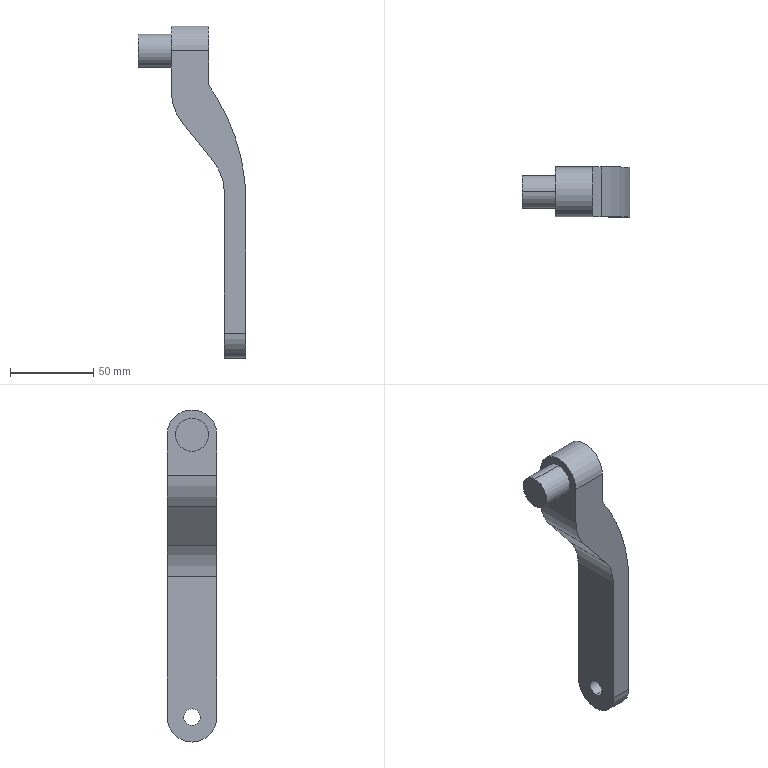Part | STEP file | Pedal LHS | 1 solid | 19 faces | box 65 x 30 x 200 mm | volume 107612 mm3 | cylinder 10 | plane 9 | commonest cylinder face diameters 30 x3 10 x2 20 x2 60 x2 240 x1
STEP:
#1=CARTESIAN_POINT('',(0.,0.,0.));
#2=DIRECTION('',(0.,0.,1.));
#3=DIRECTION('',(1.,0.,0.));
#4=AXIS2_PLACEMENT_3D('',#1,#2,#3);
#5=CARTESIAN_POINT('',(-65.,0.,10.));
#6=VERTEX_POINT('',#5);
#7=CARTESIAN_POINT('',(-65.,0.,-10.));
#8=VERTEX_POINT('',#7);
#9=CARTESIAN_POINT('',(-65.,0.,0.));
#10=DIRECTION('',(-1.,0.,0.));
#11=DIRECTION('',(0.,0.,1.));
#12=AXIS2_PLACEMENT_3D('',#9,#10,#11);
#13=CIRCLE('',#12,10.);
#14=CARTESIAN_POINT('',(-65.,0.,0.));
#15=DIRECTION('',(1.,0.,0.));
#16=DIRECTION('',(0.,0.,-1.));
#17=AXIS2_PLACEMENT_3D('',#14,#15,#16);
#18=CYLINDRICAL_SURFACE('',#17,10.);
#19=CARTESIAN_POINT('',(3.142,0.));
#20=DIRECTION('',(-1.,0.));
#21=VECTOR('',#20,1.);
#22=LINE('',#19,#21);
#23=(GEOMETRIC_REPRESENTATION_CONTEXT(2)PARAMETRIC_REPRESENTATION_CONTEXT()REPRESENTATION_CONTEXT('',''));
#24=DEFINITIONAL_REPRESENTATION('',(#22),#23);
#25=PCURVE('',#18,#24);
#26=CARTESIAN_POINT('',(-65.,0.,0.));
#27=DIRECTION('',(-1.,0.,0.));
#28=DIRECTION('',(0.,0.,1.));
#29=AXIS2_PLACEMENT_3D('',#26,#27,#28);
#30=PLANE('',#29);
#31=CARTESIAN_POINT('',(0.,0.));
#32=DIRECTION('',(1.,0.));
#33=AXIS2_PLACEMENT_2D('',#31,#32);
#34=CIRCLE('',#33,10.);
#35=(GEOMETRIC_REPRESENTATION_CONTEXT(2)PARAMETRIC_REPRESENTATION_CONTEXT()REPRESENTATION_CONTEXT('',''));
#36=DEFINITIONAL_REPRESENTATION('',(#34),#35);
#37=PCURVE('',#30,#36);
#38=SURFACE_CURVE('',#13,(#25,#37),.PCURVE_S1.);
#39=EDGE_CURVE('',#6,#8,#38,.T.);
#40=ORIENTED_EDGE('',*,*,#39,.F.);
#41=CARTESIAN_POINT('',(-45.,0.,10.));
#42=VERTEX_POINT('',#41);
#43=CARTESIAN_POINT('',(-65.,0.,10.));
#44=DIRECTION('',(1.,0.,0.));
#45=VECTOR('',#44,1.);
#46=LINE('',#43,#45);
#47=CARTESIAN_POINT('',(3.142,0.));
#48=DIRECTION('',(0.,1.));
#49=VECTOR('',#48,1.);
#50=LINE('',#47,#49);
#51=(GEOMETRIC_REPRESENTATION_CONTEXT(2)PARAMETRIC_REPRESENTATION_CONTEXT()REPRESENTATION_CONTEXT('',''));
#52=DEFINITIONAL_REPRESENTATION('',(#50),#51);
#53=PCURVE('',#18,#52);
#54=CARTESIAN_POINT('',(-65.,0.,0.));
#55=DIRECTION('',(1.,0.,0.));
#56=DIRECTION('',(0.,0.,-1.));
#57=AXIS2_PLACEMENT_3D('',#54,#55,#56);
#58=CYLINDRICAL_SURFACE('',#57,10.);
#59=CARTESIAN_POINT('',(3.142,0.));
#60=DIRECTION('',(0.,1.));
#61=VECTOR('',#60,1.);
#62=LINE('',#59,#61);
#63=(GEOMETRIC_REPRESENTATION_CONTEXT(2)PARAMETRIC_REPRESENTATION_CONTEXT()REPRESENTATION_CONTEXT('',''));
#64=DEFINITIONAL_REPRESENTATION('',(#62),#63);
#65=PCURVE('',#58,#64);
#66=SURFACE_CURVE('',#46,(#53,#65),.PCURVE_S1.);
#67=EDGE_CURVE('',#6,#42,#66,.T.);
#68=ORIENTED_EDGE('',*,*,#67,.T.);
#69=CARTESIAN_POINT('',(-45.,0.,-10.));
#70=VERTEX_POINT('',#69);
#71=CARTESIAN_POINT('',(-45.,0.,0.));
#72=DIRECTION('',(-1.,0.,0.));
#73=DIRECTION('',(0.,0.,-1.));
#74=AXIS2_PLACEMENT_3D('',#71,#72,#73);
#75=CIRCLE('',#74,10.);
#76=CARTESIAN_POINT('',(6.283,20.));
#77=DIRECTION('',(-1.,0.));
#78=VECTOR('',#77,1.);
#79=LINE('',#76,#78);
#80=(GEOMETRIC_REPRESENTATION_CONTEXT(2)PARAMETRIC_REPRESENTATION_CONTEXT()REPRESENTATION_CONTEXT('',''));
#81=DEFINITIONAL_REPRESENTATION('',(#79),#80);
#82=PCURVE('',#18,#81);
#83=CARTESIAN_POINT('',(-45.,0.,0.));
#84=DIRECTION('',(1.,0.,0.));
#85=DIRECTION('',(0.,0.,-1.));
#86=AXIS2_PLACEMENT_3D('',#83,#84,#85);
#87=PLANE('',#86);
#88=CARTESIAN_POINT('',(10.,0.));
#89=CARTESIAN_POINT('',(10.,-17.321));
#90=CARTESIAN_POINT('',(-5.,-8.66));
#91=CARTESIAN_POINT('',(-20.,0.));
#92=CARTESIAN_POINT('',(-5.,8.66));
#93=CARTESIAN_POINT('',(10.,17.321));
#94=CARTESIAN_POINT('',(10.,0.));
#95=(BOUNDED_CURVE()B_SPLINE_CURVE(2,(#88,#89,#90,#91,#92,#93,#94),.UNSPECIFIED.,.T.,.F.)B_SPLINE_CURVE_WITH_KNOTS((1,2,2,2,2,1),(-2.094,0.,2.094,4.189,6.283,8.378),.UNSPECIFIED.)CURVE()GEOMETRIC_REPRESENTATION_ITEM()RATIONAL_B_SPLINE_CURVE((1.,0.5,1.,0.5,1.,0.5,1.))REPRESENTATION_ITEM(''));
#96=(GEOMETRIC_REPRESENTATION_CONTEXT(2)PARAMETRIC_REPRESENTATION_CONTEXT()REPRESENTATION_CONTEXT('',''));
#97=DEFINITIONAL_REPRESENTATION('',(#95),#96);
#98=PCURVE('',#87,#97);
#99=SURFACE_CURVE('',#75,(#82,#98),.PCURVE_S1.);
#100=EDGE_CURVE('',#42,#70,#99,.T.);
#101=ORIENTED_EDGE('',*,*,#100,.T.);
#102=CARTESIAN_POINT('',(-65.,0.,-10.));
#103=DIRECTION('',(1.,0.,0.));
#104=VECTOR('',#103,1.);
#105=LINE('',#102,#104);
#106=CARTESIAN_POINT('',(0.,0.));
#107=DIRECTION('',(0.,1.));
#108=VECTOR('',#107,1.);
#109=LINE('',#106,#108);
#110=(GEOMETRIC_REPRESENTATION_CONTEXT(2)PARAMETRIC_REPRESENTATION_CONTEXT()REPRESENTATION_CONTEXT('',''));
#111=DEFINITIONAL_REPRESENTATION('',(#109),#110);
#112=PCURVE('',#18,#111);
#113=CARTESIAN_POINT('',(6.283,0.));
#114=DIRECTION('',(0.,1.));
#115=VECTOR('',#114,1.);
#116=LINE('',#113,#115);
#117=(GEOMETRIC_REPRESENTATION_CONTEXT(2)PARAMETRIC_REPRESENTATION_CONTEXT()REPRESENTATION_CONTEXT('',''));
#118=DEFINITIONAL_REPRESENTATION('',(#116),#117);
#119=PCURVE('',#58,#118);
#120=SURFACE_CURVE('',#105,(#112,#119),.PCURVE_S1.);
#121=EDGE_CURVE('',#8,#70,#120,.T.);
#122=ORIENTED_EDGE('',*,*,#121,.F.);
#123=EDGE_LOOP('',(#40,#68,#101,#122));
#124=FACE_BOUND('',#123,.T.);
#125=ADVANCED_FACE('',(#124),#18,.T.);
#126=CARTESIAN_POINT('',(-13.,0.,-175.));
#127=VERTEX_POINT('',#126);
#128=CARTESIAN_POINT('',(0.,0.,-175.));
#129=VERTEX_POINT('',#128);
#130=CARTESIAN_POINT('',(-45.,0.,-175.));
#131=DIRECTION('',(1.,0.,0.));
#132=VECTOR('',#131,1.);
#133=LINE('',#130,#132);
#134=CARTESIAN_POINT('',(-45.,0.,-170.));
#135=DIRECTION('',(1.,0.,0.));
#136=DIRECTION('',(0.,0.,-1.));
#137=AXIS2_PLACEMENT_3D('',#134,#135,#136);
#138=CYLINDRICAL_SURFACE('',#137,5.);
#139=CARTESIAN_POINT('',(6.283,0.));
#140=DIRECTION('',(0.,1.));
#141=VECTOR('',#140,1.);
#142=LINE('',#139,#141);
#143=(GEOMETRIC_REPRESENTATION_CONTEXT(2)PARAMETRIC_REPRESENTATION_CONTEXT()REPRESENTATION_CONTEXT('',''));
#144=DEFINITIONAL_REPRESENTATION('',(#142),#143);
#145=PCURVE('',#138,#144);
#146=CARTESIAN_POINT('',(-45.,0.,-170.));
#147=DIRECTION('',(1.,0.,0.));
#148=DIRECTION('',(0.,0.,-1.));
#149=AXIS2_PLACEMENT_3D('',#146,#147,#148);
#150=CYLINDRICAL_SURFACE('',#149,5.);
#151=CARTESIAN_POINT('',(0.,0.));
#152=DIRECTION('',(0.,1.));
#153=VECTOR('',#152,1.);
#154=LINE('',#151,#153);
#155=(GEOMETRIC_REPRESENTATION_CONTEXT(2)PARAMETRIC_REPRESENTATION_CONTEXT()REPRESENTATION_CONTEXT('',''));
#156=DEFINITIONAL_REPRESENTATION('',(#154),#155);
#157=PCURVE('',#150,#156);
#158=SURFACE_CURVE('',#133,(#145,#157),.PCURVE_S1.);
#159=EDGE_CURVE('',#127,#129,#158,.T.);
#160=ORIENTED_EDGE('',*,*,#159,.T.);
#161=CARTESIAN_POINT('',(0.,0.,-165.));
#162=VERTEX_POINT('',#161);
#163=CARTESIAN_POINT('',(0.,0.,-170.));
#164=DIRECTION('',(1.,0.,0.));
#165=DIRECTION('',(0.,0.,-1.));
#166=AXIS2_PLACEMENT_3D('',#163,#164,#165);
#167=CIRCLE('',#166,5.);
#168=CARTESIAN_POINT('',(0.,45.));
#169=DIRECTION('',(1.,0.));
#170=VECTOR('',#169,1.);
#171=LINE('',#168,#170);
#172=(GEOMETRIC_REPRESENTATION_CONTEXT(2)PARAMETRIC_REPRESENTATION_CONTEXT()REPRESENTATION_CONTEXT('',''));
#173=DEFINITIONAL_REPRESENTATION('',(#171),#172);
#174=PCURVE('',#138,#173);
#175=CARTESIAN_POINT('',(0.,0.,0.));
#176=DIRECTION('',(1.,0.,0.));
#177=DIRECTION('',(0.,0.,-1.));
#178=AXIS2_PLACEMENT_3D('',#175,#176,#177);
#179=PLANE('',#178);
#180=CARTESIAN_POINT('',(170.,0.));
#181=DIRECTION('',(1.,0.));
#182=AXIS2_PLACEMENT_2D('',#180,#181);
#183=CIRCLE('',#182,5.);
#184=(GEOMETRIC_REPRESENTATION_CONTEXT(2)PARAMETRIC_REPRESENTATION_CONTEXT()REPRESENTATION_CONTEXT('',''));
#185=DEFINITIONAL_REPRESENTATION('',(#183),#184);
#186=PCURVE('',#179,#185);
#187=SURFACE_CURVE('',#167,(#174,#186),.PCURVE_S1.);
#188=EDGE_CURVE('',#162,#129,#187,.T.);
#189=ORIENTED_EDGE('',*,*,#188,.F.);
#190=CARTESIAN_POINT('',(-13.,0.,-165.));
#191=VERTEX_POINT('',#190);
#192=CARTESIAN_POINT('',(-45.,0.,-165.));
#193=DIRECTION('',(1.,0.,0.));
#194=VECTOR('',#193,1.);
#195=LINE('',#192,#194);
#196=CARTESIAN_POINT('',(3.142,0.));
#197=DIRECTION('',(0.,1.));
#198=VECTOR('',#197,1.);
#199=LINE('',#196,#198);
#200=(GEOMETRIC_REPRESENTATION_CONTEXT(2)PARAMETRIC_REPRESENTATION_CONTEXT()REPRESENTATION_CONTEXT('',''));
#201=DEFINITIONAL_REPRESENTATION('',(#199),#200);
#202=PCURVE('',#138,#201);
#203=CARTESIAN_POINT('',(3.142,0.));
#204=DIRECTION('',(0.,1.));
#205=VECTOR('',#204,1.);
#206=LINE('',#203,#205);
#207=(GEOMETRIC_REPRESENTATION_CONTEXT(2)PARAMETRIC_REPRESENTATION_CONTEXT()REPRESENTATION_CONTEXT('',''));
#208=DEFINITIONAL_REPRESENTATION('',(#206),#207);
#209=PCURVE('',#150,#208);
#210=SURFACE_CURVE('',#195,(#202,#209),.PCURVE_S1.);
#211=EDGE_CURVE('',#191,#162,#210,.T.);
#212=ORIENTED_EDGE('',*,*,#211,.F.);
#213=CARTESIAN_POINT('',(-13.,0.,-170.));
#214=DIRECTION('',(1.,0.,0.));
#215=DIRECTION('',(0.,0.,1.));
#216=AXIS2_PLACEMENT_3D('',#213,#214,#215);
#217=CIRCLE('',#216,5.);
#218=CARTESIAN_POINT('',(3.142,32.));
#219=DIRECTION('',(1.,0.));
#220=VECTOR('',#219,1.);
#221=LINE('',#218,#220);
#222=(GEOMETRIC_REPRESENTATION_CONTEXT(2)PARAMETRIC_REPRESENTATION_CONTEXT()REPRESENTATION_CONTEXT('',''));
#223=DEFINITIONAL_REPRESENTATION('',(#221),#222);
#224=PCURVE('',#138,#223);
#225=CARTESIAN_POINT('',(-13.,-22.5,-185.));
#226=DIRECTION('',(-1.,0.,0.));
#227=DIRECTION('',(0.,0.,1.));
#228=AXIS2_PLACEMENT_3D('',#225,#226,#227);
#229=PLANE('',#228);
#230=CARTESIAN_POINT('',(20.,22.5));
#231=CARTESIAN_POINT('',(20.,13.84));
#232=CARTESIAN_POINT('',(12.5,18.17));
#233=CARTESIAN_POINT('',(5.,22.5));
#234=CARTESIAN_POINT('',(12.5,26.83));
#235=CARTESIAN_POINT('',(20.,31.16));
#236=CARTESIAN_POINT('',(20.,22.5));
#237=(BOUNDED_CURVE()B_SPLINE_CURVE(2,(#230,#231,#232,#233,#234,#235,#236),.UNSPECIFIED.,.T.,.F.)B_SPLINE_CURVE_WITH_KNOTS((1,2,2,2,2,1),(-2.094,0.,2.094,4.189,6.283,8.378),.UNSPECIFIED.)CURVE()GEOMETRIC_REPRESENTATION_ITEM()RATIONAL_B_SPLINE_CURVE((1.,0.5,1.,0.5,1.,0.5,1.))REPRESENTATION_ITEM(''));
#238=(GEOMETRIC_REPRESENTATION_CONTEXT(2)PARAMETRIC_REPRESENTATION_CONTEXT()REPRESENTATION_CONTEXT('',''));
#239=DEFINITIONAL_REPRESENTATION('',(#237),#238);
#240=PCURVE('',#229,#239);
#241=SURFACE_CURVE('',#217,(#224,#240),.PCURVE_S1.);
#242=EDGE_CURVE('',#191,#127,#241,.T.);
#243=ORIENTED_EDGE('',*,*,#242,.T.);
#244=EDGE_LOOP('',(#160,#189,#212,#243));
#245=FACE_BOUND('',#244,.F.);
#246=ADVANCED_FACE('',(#245),#138,.F.);
#247=CARTESIAN_POINT('',(-13.,-15.,-170.));
#248=VERTEX_POINT('',#247);
#249=CARTESIAN_POINT('',(-13.,0.,-185.));
#250=VERTEX_POINT('',#249);
#251=CARTESIAN_POINT('',(-13.,0.,-170.));
#252=DIRECTION('',(1.,0.,0.));
#253=DIRECTION('',(0.,0.,1.));
#254=AXIS2_PLACEMENT_3D('',#251,#252,#253);
#255=CIRCLE('',#254,15.);
#256=CARTESIAN_POINT('',(-45.,0.,-170.));
#257=DIRECTION('',(1.,0.,0.));
#258=DIRECTION('',(0.,0.,-1.));
#259=AXIS2_PLACEMENT_3D('',#256,#257,#258);
#260=CYLINDRICAL_SURFACE('',#259,15.);
#261=CARTESIAN_POINT('',(3.142,32.));
#262=DIRECTION('',(1.,0.));
#263=VECTOR('',#262,1.);
#264=LINE('',#261,#263);
#265=(GEOMETRIC_REPRESENTATION_CONTEXT(2)PARAMETRIC_REPRESENTATION_CONTEXT()REPRESENTATION_CONTEXT('',''));
#266=DEFINITIONAL_REPRESENTATION('',(#264),#265);
#267=PCURVE('',#260,#266);
#268=CARTESIAN_POINT('',(30.,22.5));
#269=CARTESIAN_POINT('',(30.,-3.481));
#270=CARTESIAN_POINT('',(7.5,9.51));
#271=CARTESIAN_POINT('',(-15.,22.5));
#272=CARTESIAN_POINT('',(7.5,35.49));
#273=CARTESIAN_POINT('',(30.,48.481));
#274=CARTESIAN_POINT('',(30.,22.5));
#275=(BOUNDED_CURVE()B_SPLINE_CURVE(2,(#268,#269,#270,#271,#272,#273,#274),.UNSPECIFIED.,.T.,.F.)B_SPLINE_CURVE_WITH_KNOTS((1,2,2,2,2,1),(-2.094,0.,2.094,4.189,6.283,8.378),.UNSPECIFIED.)CURVE()GEOMETRIC_REPRESENTATION_ITEM()RATIONAL_B_SPLINE_CURVE((1.,0.5,1.,0.5,1.,0.5,1.))REPRESENTATION_ITEM(''));
#276=(GEOMETRIC_REPRESENTATION_CONTEXT(2)PARAMETRIC_REPRESENTATION_CONTEXT()REPRESENTATION_CONTEXT('',''));
#277=DEFINITIONAL_REPRESENTATION('',(#275),#276);
#278=PCURVE('',#229,#277);
#279=SURFACE_CURVE('',#255,(#267,#278),.PCURVE_S1.);
#280=EDGE_CURVE('',#248,#250,#279,.T.);
#281=ORIENTED_EDGE('',*,*,#280,.T.);
#282=CARTESIAN_POINT('',(0.,0.,-185.));
#283=VERTEX_POINT('',#282);
#284=CARTESIAN_POINT('',(-45.,0.,-185.));
#285=DIRECTION('',(1.,0.,0.));
#286=VECTOR('',#285,1.);
#287=LINE('',#284,#286);
#288=CARTESIAN_POINT('',(6.283,0.));
#289=DIRECTION('',(0.,1.));
#290=VECTOR('',#289,1.);
#291=LINE('',#288,#290);
#292=(GEOMETRIC_REPRESENTATION_CONTEXT(2)PARAMETRIC_REPRESENTATION_CONTEXT()REPRESENTATION_CONTEXT('',''));
#293=DEFINITIONAL_REPRESENTATION('',(#291),#292);
#294=PCURVE('',#260,#293);
#295=CARTESIAN_POINT('',(-45.,0.,-170.));
#296=DIRECTION('',(1.,0.,0.));
#297=DIRECTION('',(0.,0.,-1.));
#298=AXIS2_PLACEMENT_3D('',#295,#296,#297);
#299=CYLINDRICAL_SURFACE('',#298,15.);
#300=CARTESIAN_POINT('',(0.,0.));
#301=DIRECTION('',(0.,1.));
#302=VECTOR('',#301,1.);
#303=LINE('',#300,#302);
#304=(GEOMETRIC_REPRESENTATION_CONTEXT(2)PARAMETRIC_REPRESENTATION_CONTEXT()REPRESENTATION_CONTEXT('',''));
#305=DEFINITIONAL_REPRESENTATION('',(#303),#304);
#306=PCURVE('',#299,#305);
#307=SURFACE_CURVE('',#287,(#294,#306),.PCURVE_S1.);
#308=EDGE_CURVE('',#250,#283,#307,.T.);
#309=ORIENTED_EDGE('',*,*,#308,.T.);
#310=CARTESIAN_POINT('',(0.,-15.,-170.));
#311=VERTEX_POINT('',#310);
#312=CARTESIAN_POINT('',(0.,0.,-170.));
#313=DIRECTION('',(1.,0.,0.));
#314=DIRECTION('',(0.,0.,-1.));
#315=AXIS2_PLACEMENT_3D('',#312,#313,#314);
#316=CIRCLE('',#315,15.);
#317=CARTESIAN_POINT('',(0.,45.));
#318=DIRECTION('',(1.,0.));
#319=VECTOR('',#318,1.);
#320=LINE('',#317,#319);
#321=(GEOMETRIC_REPRESENTATION_CONTEXT(2)PARAMETRIC_REPRESENTATION_CONTEXT()REPRESENTATION_CONTEXT('',''));
#322=DEFINITIONAL_REPRESENTATION('',(#320),#321);
#323=PCURVE('',#260,#322);
#324=CARTESIAN_POINT('',(170.,0.));
#325=DIRECTION('',(1.,0.));
#326=AXIS2_PLACEMENT_2D('',#324,#325);
#327=CIRCLE('',#326,15.);
#328=(GEOMETRIC_REPRESENTATION_CONTEXT(2)PARAMETRIC_REPRESENTATION_CONTEXT()REPRESENTATION_CONTEXT('',''));
#329=DEFINITIONAL_REPRESENTATION('',(#327),#328);
#330=PCURVE('',#179,#329);
#331=SURFACE_CURVE('',#316,(#323,#330),.PCURVE_S1.);
#332=EDGE_CURVE('',#311,#283,#331,.T.);
#333=ORIENTED_EDGE('',*,*,#332,.F.);
#334=CARTESIAN_POINT('',(-45.,-15.,-170.));
#335=DIRECTION('',(1.,0.,0.));
#336=VECTOR('',#335,1.);
#337=LINE('',#334,#336);
#338=CARTESIAN_POINT('',(4.712,0.));
#339=DIRECTION('',(0.,1.));
#340=VECTOR('',#339,1.);
#341=LINE('',#338,#340);
#342=(GEOMETRIC_REPRESENTATION_CONTEXT(2)PARAMETRIC_REPRESENTATION_CONTEXT()REPRESENTATION_CONTEXT('',''));
#343=DEFINITIONAL_REPRESENTATION('',(#341),#342);
#344=PCURVE('',#260,#343);
#345=CARTESIAN_POINT('',(-45.,-15.,0.));
#346=DIRECTION('',(0.,-1.,0.));
#347=DIRECTION('',(0.,0.,-1.));
#348=AXIS2_PLACEMENT_3D('',#345,#346,#347);
#349=PLANE('',#348);
#350=CARTESIAN_POINT('',(170.,0.));
#351=DIRECTION('',(0.,1.));
#352=VECTOR('',#351,1.);
#353=LINE('',#350,#352);
#354=(GEOMETRIC_REPRESENTATION_CONTEXT(2)PARAMETRIC_REPRESENTATION_CONTEXT()REPRESENTATION_CONTEXT('',''));
#355=DEFINITIONAL_REPRESENTATION('',(#353),#354);
#356=PCURVE('',#349,#355);
#357=SURFACE_CURVE('',#337,(#344,#356),.PCURVE_S1.);
#358=EDGE_CURVE('',#248,#311,#357,.T.);
#359=ORIENTED_EDGE('',*,*,#358,.F.);
#360=EDGE_LOOP('',(#281,#309,#333,#359));
#361=FACE_BOUND('',#360,.T.);
#362=ADVANCED_FACE('',(#361),#260,.T.);
#363=CARTESIAN_POINT('',(-45.,15.,-24.477));
#364=VERTEX_POINT('',#363);
#365=CARTESIAN_POINT('',(-45.,15.,0.));
#366=VERTEX_POINT('',#365);
#367=CARTESIAN_POINT('',(-45.,15.,0.));
#368=DIRECTION('',(0.,0.,1.));
#369=VECTOR('',#368,1.);
#370=LINE('',#367,#369);
#371=CARTESIAN_POINT('',(0.,15.));
#372=DIRECTION('',(-1.,0.));
#373=VECTOR('',#372,1.);
#374=LINE('',#371,#373);
#375=(GEOMETRIC_REPRESENTATION_CONTEXT(2)PARAMETRIC_REPRESENTATION_CONTEXT()REPRESENTATION_CONTEXT('',''));
#376=DEFINITIONAL_REPRESENTATION('',(#374),#375);
#377=PCURVE('',#87,#376);
#378=CARTESIAN_POINT('',(-45.,15.,0.));
#379=DIRECTION('',(0.,1.,0.));
#380=DIRECTION('',(0.,0.,1.));
#381=AXIS2_PLACEMENT_3D('',#378,#379,#380);
#382=PLANE('',#381);
#383=CARTESIAN_POINT('',(0.,0.));
#384=DIRECTION('',(1.,0.));
#385=VECTOR('',#384,1.);
#386=LINE('',#383,#385);
#387=(GEOMETRIC_REPRESENTATION_CONTEXT(2)PARAMETRIC_REPRESENTATION_CONTEXT()REPRESENTATION_CONTEXT('',''));
#388=DEFINITIONAL_REPRESENTATION('',(#386),#387);
#389=PCURVE('',#382,#388);
#390=SURFACE_CURVE('',#370,(#377,#389),.PCURVE_S1.);
#391=EDGE_CURVE('',#364,#366,#390,.T.);
#392=ORIENTED_EDGE('',*,*,#391,.F.);
#393=CARTESIAN_POINT('',(-45.,-15.,-24.477));
#394=VERTEX_POINT('',#393);
#395=CARTESIAN_POINT('',(-45.,-15.,-24.477));
#396=DIRECTION('',(0.,-1.,0.));
#397=VECTOR('',#396,1.);
#398=LINE('',#395,#397);
#399=CARTESIAN_POINT('',(24.477,-15.));
#400=DIRECTION('',(0.,-1.));
#401=VECTOR('',#400,1.);
#402=LINE('',#399,#401);
#403=(GEOMETRIC_REPRESENTATION_CONTEXT(2)PARAMETRIC_REPRESENTATION_CONTEXT()REPRESENTATION_CONTEXT('',''));
#404=DEFINITIONAL_REPRESENTATION('',(#402),#403);
#405=PCURVE('',#87,#404);
#406=CARTESIAN_POINT('',(-15.,-22.5,-24.477));
#407=DIRECTION('',(0.,-1.,0.));
#408=DIRECTION('',(0.,0.,-1.));
#409=AXIS2_PLACEMENT_3D('',#406,#407,#408);
#410=CYLINDRICAL_SURFACE('',#409,30.);
#411=CARTESIAN_POINT('',(4.712,-7.5));
#412=DIRECTION('',(0.,1.));
#413=VECTOR('',#412,1.);
#414=LINE('',#411,#413);
#415=(GEOMETRIC_REPRESENTATION_CONTEXT(2)PARAMETRIC_REPRESENTATION_CONTEXT()REPRESENTATION_CONTEXT('',''));
#416=DEFINITIONAL_REPRESENTATION('',(#414),#415);
#417=PCURVE('',#410,#416);
#418=SURFACE_CURVE('',#398,(#405,#417),.PCURVE_S1.);
#419=EDGE_CURVE('',#364,#394,#418,.T.);
#420=ORIENTED_EDGE('',*,*,#419,.T.);
#421=CARTESIAN_POINT('',(-45.,-15.,0.));
#422=VERTEX_POINT('',#421);
#423=CARTESIAN_POINT('',(-45.,-15.,0.));
#424=DIRECTION('',(0.,0.,-1.));
#425=VECTOR('',#424,1.);
#426=LINE('',#423,#425);
#427=CARTESIAN_POINT('',(0.,-15.));
#428=DIRECTION('',(1.,0.));
#429=VECTOR('',#428,1.);
#430=LINE('',#427,#429);
#431=(GEOMETRIC_REPRESENTATION_CONTEXT(2)PARAMETRIC_REPRESENTATION_CONTEXT()REPRESENTATION_CONTEXT('',''));
#432=DEFINITIONAL_REPRESENTATION('',(#430),#431);
#433=PCURVE('',#87,#432);
#434=CARTESIAN_POINT('',(0.,0.));
#435=DIRECTION('',(1.,0.));
#436=VECTOR('',#435,1.);
#437=LINE('',#434,#436);
#438=(GEOMETRIC_REPRESENTATION_CONTEXT(2)PARAMETRIC_REPRESENTATION_CONTEXT()REPRESENTATION_CONTEXT('',''));
#439=DEFINITIONAL_REPRESENTATION('',(#437),#438);
#440=PCURVE('',#349,#439);
#441=SURFACE_CURVE('',#426,(#433,#440),.PCURVE_S1.);
#442=EDGE_CURVE('',#422,#394,#441,.T.);
#443=ORIENTED_EDGE('',*,*,#442,.F.);
#444=CARTESIAN_POINT('',(-45.,0.,0.));
#445=DIRECTION('',(1.,0.,0.));
#446=DIRECTION('',(0.,0.,-1.));
#447=AXIS2_PLACEMENT_3D('',#444,#445,#446);
#448=CIRCLE('',#447,15.);
#449=CARTESIAN_POINT('',(0.,0.));
#450=DIRECTION('',(1.,0.));
#451=AXIS2_PLACEMENT_2D('',#449,#450);
#452=CIRCLE('',#451,15.);
#453=(GEOMETRIC_REPRESENTATION_CONTEXT(2)PARAMETRIC_REPRESENTATION_CONTEXT()REPRESENTATION_CONTEXT('',''));
#454=DEFINITIONAL_REPRESENTATION('',(#452),#453);
#455=PCURVE('',#87,#454);
#456=CARTESIAN_POINT('',(-45.,0.,0.));
#457=DIRECTION('',(1.,0.,0.));
#458=DIRECTION('',(0.,0.,-1.));
#459=AXIS2_PLACEMENT_3D('',#456,#457,#458);
#460=CYLINDRICAL_SURFACE('',#459,15.);
#461=CARTESIAN_POINT('',(0.,0.));
#462=DIRECTION('',(1.,0.));
#463=VECTOR('',#462,1.);
#464=LINE('',#461,#463);
#465=(GEOMETRIC_REPRESENTATION_CONTEXT(2)PARAMETRIC_REPRESENTATION_CONTEXT()REPRESENTATION_CONTEXT('',''));
#466=DEFINITIONAL_REPRESENTATION('',(#464),#465);
#467=PCURVE('',#460,#466);
#468=SURFACE_CURVE('',#448,(#455,#467),.PCURVE_S1.);
#469=EDGE_CURVE('',#366,#422,#468,.T.);
#470=ORIENTED_EDGE('',*,*,#469,.F.);
#471=EDGE_LOOP('',(#392,#420,#443,#470));
#472=FACE_BOUND('',#471,.T.);
#473=CARTESIAN_POINT('',(-45.,0.,0.));
#474=DIRECTION('',(-1.,0.,0.));
#475=DIRECTION('',(0.,0.,-1.));
#476=AXIS2_PLACEMENT_3D('',#473,#474,#475);
#477=CIRCLE('',#476,10.);
#478=CARTESIAN_POINT('',(10.,0.));
#479=CARTESIAN_POINT('',(10.,-17.321));
#480=CARTESIAN_POINT('',(-5.,-8.66));
#481=CARTESIAN_POINT('',(-20.,0.));
#482=CARTESIAN_POINT('',(-5.,8.66));
#483=CARTESIAN_POINT('',(10.,17.321));
#484=CARTESIAN_POINT('',(10.,0.));
#485=(BOUNDED_CURVE()B_SPLINE_CURVE(2,(#478,#479,#480,#481,#482,#483,#484),.UNSPECIFIED.,.T.,.F.)B_SPLINE_CURVE_WITH_KNOTS((1,2,2,2,2,1),(-2.094,0.,2.094,4.189,6.283,8.378),.UNSPECIFIED.)CURVE()GEOMETRIC_REPRESENTATION_ITEM()RATIONAL_B_SPLINE_CURVE((1.,0.5,1.,0.5,1.,0.5,1.))REPRESENTATION_ITEM(''));
#486=(GEOMETRIC_REPRESENTATION_CONTEXT(2)PARAMETRIC_REPRESENTATION_CONTEXT()REPRESENTATION_CONTEXT('',''));
#487=DEFINITIONAL_REPRESENTATION('',(#485),#486);
#488=PCURVE('',#87,#487);
#489=CARTESIAN_POINT('',(6.283,20.));
#490=DIRECTION('',(-1.,0.));
#491=VECTOR('',#490,1.);
#492=LINE('',#489,#491);
#493=(GEOMETRIC_REPRESENTATION_CONTEXT(2)PARAMETRIC_REPRESENTATION_CONTEXT()REPRESENTATION_CONTEXT('',''));
#494=DEFINITIONAL_REPRESENTATION('',(#492),#493);
#495=PCURVE('',#58,#494);
#496=SURFACE_CURVE('',#477,(#488,#495),.PCURVE_S1.);
#497=EDGE_CURVE('',#70,#42,#496,.T.);
#498=ORIENTED_EDGE('',*,*,#497,.F.);
#499=ORIENTED_EDGE('',*,*,#100,.F.);
#500=EDGE_LOOP('',(#498,#499));
#501=FACE_BOUND('',#500,.T.);
#502=ADVANCED_FACE('',(#472,#501),#87,.F.);
#503=CARTESIAN_POINT('',(-22.5,-15.,0.));
#504=VERTEX_POINT('',#503);
#505=CARTESIAN_POINT('',(-45.,-15.,0.));
#506=DIRECTION('',(1.,0.,0.));
#507=VECTOR('',#506,1.);
#508=LINE('',#505,#507);
#509=CARTESIAN_POINT('',(4.712,0.));
#510=DIRECTION('',(0.,1.));
#511=VECTOR('',#510,1.);
#512=LINE('',#509,#511);
#513=(GEOMETRIC_REPRESENTATION_CONTEXT(2)PARAMETRIC_REPRESENTATION_CONTEXT()REPRESENTATION_CONTEXT('',''));
#514=DEFINITIONAL_REPRESENTATION('',(#512),#513);
#515=PCURVE('',#460,#514);
#516=CARTESIAN_POINT('',(0.,0.));
#517=DIRECTION('',(0.,1.));
#518=VECTOR('',#517,1.);
#519=LINE('',#516,#518);
#520=(GEOMETRIC_REPRESENTATION_CONTEXT(2)PARAMETRIC_REPRESENTATION_CONTEXT()REPRESENTATION_CONTEXT('',''));
#521=DEFINITIONAL_REPRESENTATION('',(#519),#520);
#522=PCURVE('',#349,#521);
#523=SURFACE_CURVE('',#508,(#515,#522),.PCURVE_S1.);
#524=EDGE_CURVE('',#422,#504,#523,.T.);
#525=ORIENTED_EDGE('',*,*,#524,.T.);
#526=CARTESIAN_POINT('',(-22.5,15.,0.));
#527=VERTEX_POINT('',#526);
#528=CARTESIAN_POINT('',(-22.5,0.,0.));
#529=DIRECTION('',(-1.,0.,0.));
#530=DIRECTION('',(0.,0.,-1.));
#531=AXIS2_PLACEMENT_3D('',#528,#529,#530);
#532=CIRCLE('',#531,15.);
#533=CARTESIAN_POINT('',(6.283,22.5));
#534=DIRECTION('',(-1.,0.));
#535=VECTOR('',#534,1.);
#536=LINE('',#533,#535);
#537=(GEOMETRIC_REPRESENTATION_CONTEXT(2)PARAMETRIC_REPRESENTATION_CONTEXT()REPRESENTATION_CONTEXT('',''));
#538=DEFINITIONAL_REPRESENTATION('',(#536),#537);
#539=PCURVE('',#460,#538);
#540=CARTESIAN_POINT('',(-22.5,-22.5,15.));
#541=DIRECTION('',(1.,0.,0.));
#542=DIRECTION('',(0.,0.,-1.));
#543=AXIS2_PLACEMENT_3D('',#540,#541,#542);
#544=PLANE('',#543);
#545=CARTESIAN_POINT('',(30.,22.5));
#546=CARTESIAN_POINT('',(30.,-3.481));
#547=CARTESIAN_POINT('',(7.5,9.51));
#548=CARTESIAN_POINT('',(-15.,22.5));
#549=CARTESIAN_POINT('',(7.5,35.49));
#550=CARTESIAN_POINT('',(30.,48.481));
#551=CARTESIAN_POINT('',(30.,22.5));
#552=(BOUNDED_CURVE()B_SPLINE_CURVE(2,(#545,#546,#547,#548,#549,#550,#551),.UNSPECIFIED.,.T.,.F.)B_SPLINE_CURVE_WITH_KNOTS((1,2,2,2,2,1),(-2.094,0.,2.094,4.189,6.283,8.378),.UNSPECIFIED.)CURVE()GEOMETRIC_REPRESENTATION_ITEM()RATIONAL_B_SPLINE_CURVE((1.,0.5,1.,0.5,1.,0.5,1.))REPRESENTATION_ITEM(''));
#553=(GEOMETRIC_REPRESENTATION_CONTEXT(2)PARAMETRIC_REPRESENTATION_CONTEXT()REPRESENTATION_CONTEXT('',''));
#554=DEFINITIONAL_REPRESENTATION('',(#552),#553);
#555=PCURVE('',#544,#554);
#556=SURFACE_CURVE('',#532,(#539,#555),.PCURVE_S1.);
#557=EDGE_CURVE('',#504,#527,#556,.T.);
#558=ORIENTED_EDGE('',*,*,#557,.T.);
#559=CARTESIAN_POINT('',(-45.,15.,0.));
#560=DIRECTION('',(1.,0.,0.));
#561=VECTOR('',#560,1.);
#562=LINE('',#559,#561);
#563=CARTESIAN_POINT('',(1.571,0.));
#564=DIRECTION('',(0.,1.));
#565=VECTOR('',#564,1.);
#566=LINE('',#563,#565);
#567=(GEOMETRIC_REPRESENTATION_CONTEXT(2)PARAMETRIC_REPRESENTATION_CONTEXT()REPRESENTATION_CONTEXT('',''));
#568=DEFINITIONAL_REPRESENTATION('',(#566),#567);
#569=PCURVE('',#460,#568);
#570=CARTESIAN_POINT('',(0.,0.));
#571=DIRECTION('',(0.,1.));
#572=VECTOR('',#571,1.);
#573=LINE('',#570,#572);
#574=(GEOMETRIC_REPRESENTATION_CONTEXT(2)PARAMETRIC_REPRESENTATION_CONTEXT()REPRESENTATION_CONTEXT('',''));
#575=DEFINITIONAL_REPRESENTATION('',(#573),#574);
#576=PCURVE('',#382,#575);
#577=SURFACE_CURVE('',#562,(#569,#576),.PCURVE_S1.);
#578=EDGE_CURVE('',#366,#527,#577,.T.);
#579=ORIENTED_EDGE('',*,*,#578,.F.);
#580=ORIENTED_EDGE('',*,*,#469,.T.);
#581=EDGE_LOOP('',(#525,#558,#579,#580));
#582=FACE_BOUND('',#581,.T.);
#583=ADVANCED_FACE('',(#582),#460,.T.);
#584=CARTESIAN_POINT('',(-22.5,15.,-20.4));
#585=VERTEX_POINT('',#584);
#586=CARTESIAN_POINT('',(-17.395,15.,-28.818));
#587=VERTEX_POINT('',#586);
#588=CARTESIAN_POINT('',(-37.595,15.,4.491));
#589=DIRECTION('',(0.5186,0.,-0.855));
#590=VECTOR('',#589,1.);
#591=LINE('',#588,#590);
#592=CARTESIAN_POINT('',(4.491,7.405));
#593=DIRECTION('',(-0.855,0.5186));
#594=VECTOR('',#593,1.);
#595=LINE('',#592,#594);
#596=(GEOMETRIC_REPRESENTATION_CONTEXT(2)PARAMETRIC_REPRESENTATION_CONTEXT()REPRESENTATION_CONTEXT('',''));
#597=DEFINITIONAL_REPRESENTATION('',(#595),#596);
#598=PCURVE('',#382,#597);
#599=CARTESIAN_POINT('',(-22.5,-22.5,-20.4));
#600=DIRECTION('',(0.855,0.,0.5186));
#601=DIRECTION('',(0.5186,0.,-0.855));
#602=AXIS2_PLACEMENT_3D('',#599,#600,#601);
#603=PLANE('',#602);
#604=CARTESIAN_POINT('',(-29.11,37.5));
#605=DIRECTION('',(1.,0.));
#606=VECTOR('',#605,1.);
#607=LINE('',#604,#606);
#608=(GEOMETRIC_REPRESENTATION_CONTEXT(2)PARAMETRIC_REPRESENTATION_CONTEXT()REPRESENTATION_CONTEXT('',''));
#609=DEFINITIONAL_REPRESENTATION('',(#607),#608);
#610=PCURVE('',#603,#609);
#611=SURFACE_CURVE('',#591,(#598,#610),.PCURVE_S1.);
#612=EDGE_CURVE('',#585,#587,#611,.T.);
#613=ORIENTED_EDGE('',*,*,#612,.T.);
#614=CARTESIAN_POINT('',(0.,15.,-91.044));
#615=VERTEX_POINT('',#614);
#616=CARTESIAN_POINT('',(-120.,15.,-91.044));
#617=DIRECTION('',(0.,1.,0.));
#618=DIRECTION('',(0.,0.,1.));
#619=AXIS2_PLACEMENT_3D('',#616,#617,#618);
#620=CIRCLE('',#619,120.);
#621=CARTESIAN_POINT('',(-91.044,-75.));
#622=DIRECTION('',(1.,0.));
#623=AXIS2_PLACEMENT_2D('',#621,#622);
#624=CIRCLE('',#623,120.);
#625=(GEOMETRIC_REPRESENTATION_CONTEXT(2)PARAMETRIC_REPRESENTATION_CONTEXT()REPRESENTATION_CONTEXT('',''));
#626=DEFINITIONAL_REPRESENTATION('',(#624),#625);
#627=PCURVE('',#382,#626);
#628=CARTESIAN_POINT('',(-120.,-22.5,-91.044));
#629=DIRECTION('',(0.,1.,0.));
#630=DIRECTION('',(0.,0.,1.));
#631=AXIS2_PLACEMENT_3D('',#628,#629,#630);
#632=CYLINDRICAL_SURFACE('',#631,120.);
#633=CARTESIAN_POINT('',(0.,37.5));
#634=DIRECTION('',(1.,0.));
#635=VECTOR('',#634,1.);
#636=LINE('',#633,#635);
#637=(GEOMETRIC_REPRESENTATION_CONTEXT(2)PARAMETRIC_REPRESENTATION_CONTEXT()REPRESENTATION_CONTEXT('',''));
#638=DEFINITIONAL_REPRESENTATION('',(#636),#637);
#639=PCURVE('',#632,#638);
#640=SURFACE_CURVE('',#620,(#627,#639),.PCURVE_S1.);
#641=EDGE_CURVE('',#587,#615,#640,.T.);
#642=ORIENTED_EDGE('',*,*,#641,.T.);
#643=CARTESIAN_POINT('',(0.,15.,-170.));
#644=VERTEX_POINT('',#643);
#645=CARTESIAN_POINT('',(0.,15.,0.));
#646=DIRECTION('',(0.,0.,1.));
#647=VECTOR('',#646,1.);
#648=LINE('',#645,#647);
#649=CARTESIAN_POINT('',(0.,45.));
#650=DIRECTION('',(1.,0.));
#651=VECTOR('',#650,1.);
#652=LINE('',#649,#651);
#653=(GEOMETRIC_REPRESENTATION_CONTEXT(2)PARAMETRIC_REPRESENTATION_CONTEXT()REPRESENTATION_CONTEXT('',''));
#654=DEFINITIONAL_REPRESENTATION('',(#652),#653);
#655=PCURVE('',#382,#654);
#656=CARTESIAN_POINT('',(0.,15.));
#657=DIRECTION('',(-1.,0.));
#658=VECTOR('',#657,1.);
#659=LINE('',#656,#658);
#660=(GEOMETRIC_REPRESENTATION_CONTEXT(2)PARAMETRIC_REPRESENTATION_CONTEXT()REPRESENTATION_CONTEXT('',''));
#661=DEFINITIONAL_REPRESENTATION('',(#659),#660);
#662=PCURVE('',#179,#661);
#663=SURFACE_CURVE('',#648,(#655,#662),.PCURVE_S1.);
#664=EDGE_CURVE('',#644,#615,#663,.T.);
#665=ORIENTED_EDGE('',*,*,#664,.F.);
#666=CARTESIAN_POINT('',(-13.,15.,-170.));
#667=VERTEX_POINT('',#666);
#668=CARTESIAN_POINT('',(-45.,15.,-170.));
#669=DIRECTION('',(1.,0.,0.));
#670=VECTOR('',#669,1.);
#671=LINE('',#668,#670);
#672=CARTESIAN_POINT('',(-170.,0.));
#673=DIRECTION('',(0.,1.));
#674=VECTOR('',#673,1.);
#675=LINE('',#672,#674);
#676=(GEOMETRIC_REPRESENTATION_CONTEXT(2)PARAMETRIC_REPRESENTATION_CONTEXT()REPRESENTATION_CONTEXT('',''));
#677=DEFINITIONAL_REPRESENTATION('',(#675),#676);
#678=PCURVE('',#382,#677);
#679=CARTESIAN_POINT('',(1.571,0.));
#680=DIRECTION('',(0.,1.));
#681=VECTOR('',#680,1.);
#682=LINE('',#679,#681);
#683=(GEOMETRIC_REPRESENTATION_CONTEXT(2)PARAMETRIC_REPRESENTATION_CONTEXT()REPRESENTATION_CONTEXT('',''));
#684=DEFINITIONAL_REPRESENTATION('',(#682),#683);
#685=PCURVE('',#299,#684);
#686=SURFACE_CURVE('',#671,(#678,#685),.PCURVE_S1.);
#687=EDGE_CURVE('',#667,#644,#686,.T.);
#688=ORIENTED_EDGE('',*,*,#687,.F.);
#689=CARTESIAN_POINT('',(-13.,15.,-85.523));
#690=VERTEX_POINT('',#689);
#691=CARTESIAN_POINT('',(-13.,15.,0.));
#692=DIRECTION('',(0.,0.,1.));
#693=VECTOR('',#692,1.);
#694=LINE('',#691,#693);
#695=CARTESIAN_POINT('',(0.,32.));
#696=DIRECTION('',(1.,0.));
#697=VECTOR('',#696,1.);
#698=LINE('',#695,#697);
#699=(GEOMETRIC_REPRESENTATION_CONTEXT(2)PARAMETRIC_REPRESENTATION_CONTEXT()REPRESENTATION_CONTEXT('',''));
#700=DEFINITIONAL_REPRESENTATION('',(#698),#699);
#701=PCURVE('',#382,#700);
#702=CARTESIAN_POINT('',(185.,37.5));
#703=DIRECTION('',(1.,0.));
#704=VECTOR('',#703,1.);
#705=LINE('',#702,#704);
#706=(GEOMETRIC_REPRESENTATION_CONTEXT(2)PARAMETRIC_REPRESENTATION_CONTEXT()REPRESENTATION_CONTEXT('',''));
#707=DEFINITIONAL_REPRESENTATION('',(#705),#706);
#708=PCURVE('',#229,#707);
#709=SURFACE_CURVE('',#694,(#701,#708),.PCURVE_S1.);
#710=EDGE_CURVE('',#667,#690,#709,.T.);
#711=ORIENTED_EDGE('',*,*,#710,.T.);
#712=CARTESIAN_POINT('',(-19.574,15.,-66.783));
#713=VERTEX_POINT('',#712);
#714=CARTESIAN_POINT('',(-43.,15.,-85.523));
#715=DIRECTION('',(0.,-1.,0.));
#716=DIRECTION('',(0.,0.,1.));
#717=AXIS2_PLACEMENT_3D('',#714,#715,#716);
#718=CIRCLE('',#717,30.);
#719=CARTESIAN_POINT('',(-55.523,2.));
#720=CARTESIAN_POINT('',(-55.523,-49.962));
#721=CARTESIAN_POINT('',(-100.523,-23.981));
#722=CARTESIAN_POINT('',(-145.523,2.));
#723=CARTESIAN_POINT('',(-100.523,27.981));
#724=CARTESIAN_POINT('',(-55.523,53.962));
#725=CARTESIAN_POINT('',(-55.523,2.));
#726=(BOUNDED_CURVE()B_SPLINE_CURVE(2,(#719,#720,#721,#722,#723,#724,#725),.UNSPECIFIED.,.T.,.F.)B_SPLINE_CURVE_WITH_KNOTS((1,2,2,2,2,1),(-2.094,0.,2.094,4.189,6.283,8.378),.UNSPECIFIED.)CURVE()GEOMETRIC_REPRESENTATION_ITEM()RATIONAL_B_SPLINE_CURVE((1.,0.5,1.,0.5,1.,0.5,1.))REPRESENTATION_ITEM(''));
#727=(GEOMETRIC_REPRESENTATION_CONTEXT(2)PARAMETRIC_REPRESENTATION_CONTEXT()REPRESENTATION_CONTEXT('',''));
#728=DEFINITIONAL_REPRESENTATION('',(#726),#727);
#729=PCURVE('',#382,#728);
#730=CARTESIAN_POINT('',(-43.,-22.5,-85.523));
#731=DIRECTION('',(0.,-1.,0.));
#732=DIRECTION('',(0.,0.,-1.));
#733=AXIS2_PLACEMENT_3D('',#730,#731,#732);
#734=CYLINDRICAL_SURFACE('',#733,30.);
#735=CARTESIAN_POINT('',(-3.142,-37.5));
#736=DIRECTION('',(1.,0.));
#737=VECTOR('',#736,1.);
#738=LINE('',#735,#737);
#739=(GEOMETRIC_REPRESENTATION_CONTEXT(2)PARAMETRIC_REPRESENTATION_CONTEXT()REPRESENTATION_CONTEXT('',''));
#740=DEFINITIONAL_REPRESENTATION('',(#738),#739);
#741=PCURVE('',#734,#740);
#742=SURFACE_CURVE('',#718,(#729,#741),.PCURVE_S1.);
#743=EDGE_CURVE('',#690,#713,#742,.T.);
#744=ORIENTED_EDGE('',*,*,#743,.T.);
#745=CARTESIAN_POINT('',(-38.426,15.,-43.217));
#746=VERTEX_POINT('',#745);
#747=CARTESIAN_POINT('',(-62.073,15.,-13.659));
#748=DIRECTION('',(-0.6247,0.,0.7809));
#749=VECTOR('',#748,1.);
#750=LINE('',#747,#749);
#751=CARTESIAN_POINT('',(-13.659,-17.073));
#752=DIRECTION('',(0.7809,-0.6247));
#753=VECTOR('',#752,1.);
#754=LINE('',#751,#753);
#755=(GEOMETRIC_REPRESENTATION_CONTEXT(2)PARAMETRIC_REPRESENTATION_CONTEXT()REPRESENTATION_CONTEXT('',''));
#756=DEFINITIONAL_REPRESENTATION('',(#754),#755);
#757=PCURVE('',#382,#756);
#758=CARTESIAN_POINT('',(-13.,-22.5,-75.));
#759=DIRECTION('',(-0.7809,0.,-0.6247));
#760=DIRECTION('',(-0.6247,0.,0.7809));
#761=AXIS2_PLACEMENT_3D('',#758,#759,#760);
#762=PLANE('',#761);
#763=CARTESIAN_POINT('',(78.555,37.5));
#764=DIRECTION('',(1.,0.));
#765=VECTOR('',#764,1.);
#766=LINE('',#763,#765);
#767=(GEOMETRIC_REPRESENTATION_CONTEXT(2)PARAMETRIC_REPRESENTATION_CONTEXT()REPRESENTATION_CONTEXT('',''));
#768=DEFINITIONAL_REPRESENTATION('',(#766),#767);
#769=PCURVE('',#762,#768);
#770=SURFACE_CURVE('',#750,(#757,#769),.PCURVE_S1.);
#771=EDGE_CURVE('',#713,#746,#770,.T.);
#772=ORIENTED_EDGE('',*,*,#771,.T.);
#773=CARTESIAN_POINT('',(-15.,15.,-24.477));
#774=DIRECTION('',(0.,1.,0.));
#775=DIRECTION('',(0.,0.,1.));
#776=AXIS2_PLACEMENT_3D('',#773,#774,#775);
#777=CIRCLE('',#776,30.);
#778=CARTESIAN_POINT('',(-24.477,30.));
#779=DIRECTION('',(1.,0.));
#780=AXIS2_PLACEMENT_2D('',#778,#779);
#781=CIRCLE('',#780,30.);
#782=(GEOMETRIC_REPRESENTATION_CONTEXT(2)PARAMETRIC_REPRESENTATION_CONTEXT()REPRESENTATION_CONTEXT('',''));
#783=DEFINITIONAL_REPRESENTATION('',(#781),#782);
#784=PCURVE('',#382,#783);
#785=CARTESIAN_POINT('',(9.425,-37.5));
#786=DIRECTION('',(-1.,0.));
#787=VECTOR('',#786,1.);
#788=LINE('',#785,#787);
#789=(GEOMETRIC_REPRESENTATION_CONTEXT(2)PARAMETRIC_REPRESENTATION_CONTEXT()REPRESENTATION_CONTEXT('',''));
#790=DEFINITIONAL_REPRESENTATION('',(#788),#789);
#791=PCURVE('',#410,#790);
#792=SURFACE_CURVE('',#777,(#784,#791),.PCURVE_S1.);
#793=EDGE_CURVE('',#746,#364,#792,.T.);
#794=ORIENTED_EDGE('',*,*,#793,.T.);
#795=ORIENTED_EDGE('',*,*,#391,.T.);
#796=ORIENTED_EDGE('',*,*,#578,.T.);
#797=CARTESIAN_POINT('',(-22.5,15.,0.));
#798=DIRECTION('',(0.,0.,-1.));
#799=VECTOR('',#798,1.);
#800=LINE('',#797,#799);
#801=CARTESIAN_POINT('',(0.,22.5));
#802=DIRECTION('',(-1.,0.));
#803=VECTOR('',#802,1.);
#804=LINE('',#801,#803);
#805=(GEOMETRIC_REPRESENTATION_CONTEXT(2)PARAMETRIC_REPRESENTATION_CONTEXT()REPRESENTATION_CONTEXT('',''));
#806=DEFINITIONAL_REPRESENTATION('',(#804),#805);
#807=PCURVE('',#382,#806);
#808=CARTESIAN_POINT('',(15.,37.5));
#809=DIRECTION('',(1.,0.));
#810=VECTOR('',#809,1.);
#811=LINE('',#808,#810);
#812=(GEOMETRIC_REPRESENTATION_CONTEXT(2)PARAMETRIC_REPRESENTATION_CONTEXT()REPRESENTATION_CONTEXT('',''));
#813=DEFINITIONAL_REPRESENTATION('',(#811),#812);
#814=PCURVE('',#544,#813);
#815=SURFACE_CURVE('',#800,(#807,#814),.PCURVE_S1.);
#816=EDGE_CURVE('',#527,#585,#815,.T.);
#817=ORIENTED_EDGE('',*,*,#816,.T.);
#818=EDGE_LOOP('',(#613,#642,#665,#688,#711,#744,#772,#794,#795,#796,#817));
#819=FACE_BOUND('',#818,.T.);
#820=ADVANCED_FACE('',(#819),#382,.T.);
#821=ORIENTED_EDGE('',*,*,#308,.F.);
#822=CARTESIAN_POINT('',(-13.,0.,-170.));
#823=DIRECTION('',(1.,0.,0.));
#824=DIRECTION('',(0.,0.,1.));
#825=AXIS2_PLACEMENT_3D('',#822,#823,#824);
#826=CIRCLE('',#825,15.);
#827=CARTESIAN_POINT('',(-3.142,32.));
#828=DIRECTION('',(1.,0.));
#829=VECTOR('',#828,1.);
#830=LINE('',#827,#829);
#831=(GEOMETRIC_REPRESENTATION_CONTEXT(2)PARAMETRIC_REPRESENTATION_CONTEXT()REPRESENTATION_CONTEXT('',''));
#832=DEFINITIONAL_REPRESENTATION('',(#830),#831);
#833=PCURVE('',#299,#832);
#834=CARTESIAN_POINT('',(30.,22.5));
#835=CARTESIAN_POINT('',(30.,-3.481));
#836=CARTESIAN_POINT('',(7.5,9.51));
#837=CARTESIAN_POINT('',(-15.,22.5));
#838=CARTESIAN_POINT('',(7.5,35.49));
#839=CARTESIAN_POINT('',(30.,48.481));
#840=CARTESIAN_POINT('',(30.,22.5));
#841=(BOUNDED_CURVE()B_SPLINE_CURVE(2,(#834,#835,#836,#837,#838,#839,#840),.UNSPECIFIED.,.T.,.F.)B_SPLINE_CURVE_WITH_KNOTS((1,2,2,2,2,1),(-2.094,0.,2.094,4.189,6.283,8.378),.UNSPECIFIED.)CURVE()GEOMETRIC_REPRESENTATION_ITEM()RATIONAL_B_SPLINE_CURVE((1.,0.5,1.,0.5,1.,0.5,1.))REPRESENTATION_ITEM(''));
#842=(GEOMETRIC_REPRESENTATION_CONTEXT(2)PARAMETRIC_REPRESENTATION_CONTEXT()REPRESENTATION_CONTEXT('',''));
#843=DEFINITIONAL_REPRESENTATION('',(#841),#842);
#844=PCURVE('',#229,#843);
#845=SURFACE_CURVE('',#826,(#833,#844),.PCURVE_S1.);
#846=EDGE_CURVE('',#250,#667,#845,.T.);
#847=ORIENTED_EDGE('',*,*,#846,.T.);
#848=ORIENTED_EDGE('',*,*,#687,.T.);
#849=CARTESIAN_POINT('',(0.,0.,-170.));
#850=DIRECTION('',(1.,0.,0.));
#851=DIRECTION('',(0.,0.,-1.));
#852=AXIS2_PLACEMENT_3D('',#849,#850,#851);
#853=CIRCLE('',#852,15.);
#854=CARTESIAN_POINT('',(0.,45.));
#855=DIRECTION('',(1.,0.));
#856=VECTOR('',#855,1.);
#857=LINE('',#854,#856);
#858=(GEOMETRIC_REPRESENTATION_CONTEXT(2)PARAMETRIC_REPRESENTATION_CONTEXT()REPRESENTATION_CONTEXT('',''));
#859=DEFINITIONAL_REPRESENTATION('',(#857),#858);
#860=PCURVE('',#299,#859);
#861=CARTESIAN_POINT('',(170.,0.));
#862=DIRECTION('',(1.,0.));
#863=AXIS2_PLACEMENT_2D('',#861,#862);
#864=CIRCLE('',#863,15.);
#865=(GEOMETRIC_REPRESENTATION_CONTEXT(2)PARAMETRIC_REPRESENTATION_CONTEXT()REPRESENTATION_CONTEXT('',''));
#866=DEFINITIONAL_REPRESENTATION('',(#864),#865);
#867=PCURVE('',#179,#866);
#868=SURFACE_CURVE('',#853,(#860,#867),.PCURVE_S1.);
#869=EDGE_CURVE('',#283,#644,#868,.T.);
#870=ORIENTED_EDGE('',*,*,#869,.F.);
#871=EDGE_LOOP('',(#821,#847,#848,#870));
#872=FACE_BOUND('',#871,.T.);
#873=ADVANCED_FACE('',(#872),#299,.T.);
#874=CARTESIAN_POINT('',(0.,-15.,-91.044));
#875=VERTEX_POINT('',#874);
#876=CARTESIAN_POINT('',(0.,-15.,0.));
#877=DIRECTION('',(0.,0.,-1.));
#878=VECTOR('',#877,1.);
#879=LINE('',#876,#878);
#880=CARTESIAN_POINT('',(0.,45.));
#881=DIRECTION('',(1.,0.));
#882=VECTOR('',#881,1.);
#883=LINE('',#880,#882);
#884=(GEOMETRIC_REPRESENTATION_CONTEXT(2)PARAMETRIC_REPRESENTATION_CONTEXT()REPRESENTATION_CONTEXT('',''));
#885=DEFINITIONAL_REPRESENTATION('',(#883),#884);
#886=PCURVE('',#349,#885);
#887=CARTESIAN_POINT('',(0.,-15.));
#888=DIRECTION('',(1.,0.));
#889=VECTOR('',#888,1.);
#890=LINE('',#887,#889);
#891=(GEOMETRIC_REPRESENTATION_CONTEXT(2)PARAMETRIC_REPRESENTATION_CONTEXT()REPRESENTATION_CONTEXT('',''));
#892=DEFINITIONAL_REPRESENTATION('',(#890),#891);
#893=PCURVE('',#179,#892);
#894=SURFACE_CURVE('',#879,(#886,#893),.PCURVE_S1.);
#895=EDGE_CURVE('',#875,#311,#894,.T.);
#896=ORIENTED_EDGE('',*,*,#895,.F.);
#897=CARTESIAN_POINT('',(-17.395,-15.,-28.818));
#898=VERTEX_POINT('',#897);
#899=CARTESIAN_POINT('',(-120.,-15.,-91.044));
#900=DIRECTION('',(0.,-1.,0.));
#901=DIRECTION('',(0.,0.,-1.));
#902=AXIS2_PLACEMENT_3D('',#899,#900,#901);
#903=CIRCLE('',#902,120.);
#904=CARTESIAN_POINT('',(91.044,-75.));
#905=DIRECTION('',(1.,0.));
#906=AXIS2_PLACEMENT_2D('',#904,#905);
#907=CIRCLE('',#906,120.);
#908=(GEOMETRIC_REPRESENTATION_CONTEXT(2)PARAMETRIC_REPRESENTATION_CONTEXT()REPRESENTATION_CONTEXT('',''));
#909=DEFINITIONAL_REPRESENTATION('',(#907),#908);
#910=PCURVE('',#349,#909);
#911=CARTESIAN_POINT('',(3.142,7.5));
#912=DIRECTION('',(-1.,0.));
#913=VECTOR('',#912,1.);
#914=LINE('',#911,#913);
#915=(GEOMETRIC_REPRESENTATION_CONTEXT(2)PARAMETRIC_REPRESENTATION_CONTEXT()REPRESENTATION_CONTEXT('',''));
#916=DEFINITIONAL_REPRESENTATION('',(#914),#915);
#917=PCURVE('',#632,#916);
#918=SURFACE_CURVE('',#903,(#910,#917),.PCURVE_S1.);
#919=EDGE_CURVE('',#875,#898,#918,.T.);
#920=ORIENTED_EDGE('',*,*,#919,.T.);
#921=CARTESIAN_POINT('',(-22.5,-15.,-20.4));
#922=VERTEX_POINT('',#921);
#923=CARTESIAN_POINT('',(-37.595,-15.,4.491));
#924=DIRECTION('',(-0.5186,0.,0.855));
#925=VECTOR('',#924,1.);
#926=LINE('',#923,#925);
#927=CARTESIAN_POINT('',(-4.491,7.405));
#928=DIRECTION('',(-0.855,-0.5186));
#929=VECTOR('',#928,1.);
#930=LINE('',#927,#929);
#931=(GEOMETRIC_REPRESENTATION_CONTEXT(2)PARAMETRIC_REPRESENTATION_CONTEXT()REPRESENTATION_CONTEXT('',''));
#932=DEFINITIONAL_REPRESENTATION('',(#930),#931);
#933=PCURVE('',#349,#932);
#934=CARTESIAN_POINT('',(-29.11,7.5));
#935=DIRECTION('',(-1.,0.));
#936=VECTOR('',#935,1.);
#937=LINE('',#934,#936);
#938=(GEOMETRIC_REPRESENTATION_CONTEXT(2)PARAMETRIC_REPRESENTATION_CONTEXT()REPRESENTATION_CONTEXT('',''));
#939=DEFINITIONAL_REPRESENTATION('',(#937),#938);
#940=PCURVE('',#603,#939);
#941=SURFACE_CURVE('',#926,(#933,#940),.PCURVE_S1.);
#942=EDGE_CURVE('',#898,#922,#941,.T.);
#943=ORIENTED_EDGE('',*,*,#942,.T.);
#944=CARTESIAN_POINT('',(-22.5,-15.,0.));
#945=DIRECTION('',(0.,0.,1.));
#946=VECTOR('',#945,1.);
#947=LINE('',#944,#946);
#948=CARTESIAN_POINT('',(0.,22.5));
#949=DIRECTION('',(-1.,0.));
#950=VECTOR('',#949,1.);
#951=LINE('',#948,#950);
#952=(GEOMETRIC_REPRESENTATION_CONTEXT(2)PARAMETRIC_REPRESENTATION_CONTEXT()REPRESENTATION_CONTEXT('',''));
#953=DEFINITIONAL_REPRESENTATION('',(#951),#952);
#954=PCURVE('',#349,#953);
#955=CARTESIAN_POINT('',(15.,7.5));
#956=DIRECTION('',(-1.,0.));
#957=VECTOR('',#956,1.);
#958=LINE('',#955,#957);
#959=(GEOMETRIC_REPRESENTATION_CONTEXT(2)PARAMETRIC_REPRESENTATION_CONTEXT()REPRESENTATION_CONTEXT('',''));
#960=DEFINITIONAL_REPRESENTATION('',(#958),#959);
#961=PCURVE('',#544,#960);
#962=SURFACE_CURVE('',#947,(#954,#961),.PCURVE_S1.);
#963=EDGE_CURVE('',#922,#504,#962,.T.);
#964=ORIENTED_EDGE('',*,*,#963,.T.);
#965=ORIENTED_EDGE('',*,*,#524,.F.);
#966=ORIENTED_EDGE('',*,*,#442,.T.);
#967=CARTESIAN_POINT('',(-38.426,-15.,-43.217));
#968=VERTEX_POINT('',#967);
#969=CARTESIAN_POINT('',(-15.,-15.,-24.477));
#970=DIRECTION('',(0.,-1.,0.));
#971=DIRECTION('',(0.,0.,-1.));
#972=AXIS2_PLACEMENT_3D('',#969,#970,#971);
#973=CIRCLE('',#972,30.);
#974=CARTESIAN_POINT('',(24.477,30.));
#975=DIRECTION('',(1.,0.));
#976=AXIS2_PLACEMENT_2D('',#974,#975);
#977=CIRCLE('',#976,30.);
#978=(GEOMETRIC_REPRESENTATION_CONTEXT(2)PARAMETRIC_REPRESENTATION_CONTEXT()REPRESENTATION_CONTEXT('',''));
#979=DEFINITIONAL_REPRESENTATION('',(#977),#978);
#980=PCURVE('',#349,#979);
#981=CARTESIAN_POINT('',(0.,-7.5));
#982=DIRECTION('',(1.,0.));
#983=VECTOR('',#982,1.);
#984=LINE('',#981,#983);
#985=(GEOMETRIC_REPRESENTATION_CONTEXT(2)PARAMETRIC_REPRESENTATION_CONTEXT()REPRESENTATION_CONTEXT('',''));
#986=DEFINITIONAL_REPRESENTATION('',(#984),#985);
#987=PCURVE('',#410,#986);
#988=SURFACE_CURVE('',#973,(#980,#987),.PCURVE_S1.);
#989=EDGE_CURVE('',#394,#968,#988,.T.);
#990=ORIENTED_EDGE('',*,*,#989,.T.);
#991=CARTESIAN_POINT('',(-19.574,-15.,-66.783));
#992=VERTEX_POINT('',#991);
#993=CARTESIAN_POINT('',(-62.073,-15.,-13.659));
#994=DIRECTION('',(0.6247,0.,-0.7809));
#995=VECTOR('',#994,1.);
#996=LINE('',#993,#995);
#997=CARTESIAN_POINT('',(13.659,-17.073));
#998=DIRECTION('',(0.7809,0.6247));
#999=VECTOR('',#998,1.);
#1000=LINE('',#997,#999);
#1001=(GEOMETRIC_REPRESENTATION_CONTEXT(2)PARAMETRIC_REPRESENTATION_CONTEXT()REPRESENTATION_CONTEXT('',''));
#1002=DEFINITIONAL_REPRESENTATION('',(#1000),#1001);
#1003=PCURVE('',#349,#1002);
#1004=CARTESIAN_POINT('',(78.555,7.5));
#1005=DIRECTION('',(-1.,0.));
#1006=VECTOR('',#1005,1.);
#1007=LINE('',#1004,#1006);
#1008=(GEOMETRIC_REPRESENTATION_CONTEXT(2)PARAMETRIC_REPRESENTATION_CONTEXT()REPRESENTATION_CONTEXT('',''));
#1009=DEFINITIONAL_REPRESENTATION('',(#1007),#1008);
#1010=PCURVE('',#762,#1009);
#1011=SURFACE_CURVE('',#996,(#1003,#1010),.PCURVE_S1.);
#1012=EDGE_CURVE('',#968,#992,#1011,.T.);
#1013=ORIENTED_EDGE('',*,*,#1012,.T.);
#1014=CARTESIAN_POINT('',(-13.,-15.,-85.523));
#1015=VERTEX_POINT('',#1014);
#1016=CARTESIAN_POINT('',(-43.,-15.,-85.523));
#1017=DIRECTION('',(0.,1.,0.));
#1018=DIRECTION('',(0.,0.,-1.));
#1019=AXIS2_PLACEMENT_3D('',#1016,#1017,#1018);
#1020=CIRCLE('',#1019,30.);
#1021=CARTESIAN_POINT('',(115.523,2.));
#1022=CARTESIAN_POINT('',(115.523,-49.962));
#1023=CARTESIAN_POINT('',(70.523,-23.981));
#1024=CARTESIAN_POINT('',(25.523,2.));
#1025=CARTESIAN_POINT('',(70.523,27.981));
#1026=CARTESIAN_POINT('',(115.523,53.962));
#1027=CARTESIAN_POINT('',(115.523,2.));
#1028=(BOUNDED_CURVE()B_SPLINE_CURVE(2,(#1021,#1022,#1023,#1024,#1025,#1026,#1027),.UNSPECIFIED.,.T.,.F.)B_SPLINE_CURVE_WITH_KNOTS((1,2,2,2,2,1),(-2.094,0.,2.094,4.189,6.283,8.378),.UNSPECIFIED.)CURVE()GEOMETRIC_REPRESENTATION_ITEM()RATIONAL_B_SPLINE_CURVE((1.,0.5,1.,0.5,1.,0.5,1.))REPRESENTATION_ITEM(''));
#1029=(GEOMETRIC_REPRESENTATION_CONTEXT(2)PARAMETRIC_REPRESENTATION_CONTEXT()REPRESENTATION_CONTEXT('',''));
#1030=DEFINITIONAL_REPRESENTATION('',(#1028),#1029);
#1031=PCURVE('',#349,#1030);
#1032=CARTESIAN_POINT('',(6.283,-7.5));
#1033=DIRECTION('',(-1.,0.));
#1034=VECTOR('',#1033,1.);
#1035=LINE('',#1032,#1034);
#1036=(GEOMETRIC_REPRESENTATION_CONTEXT(2)PARAMETRIC_REPRESENTATION_CONTEXT()REPRESENTATION_CONTEXT('',''));
#1037=DEFINITIONAL_REPRESENTATION('',(#1035),#1036);
#1038=PCURVE('',#734,#1037);
#1039=SURFACE_CURVE('',#1020,(#1031,#1038),.PCURVE_S1.);
#1040=EDGE_CURVE('',#992,#1015,#1039,.T.);
#1041=ORIENTED_EDGE('',*,*,#1040,.T.);
#1042=CARTESIAN_POINT('',(-13.,-15.,0.));
#1043=DIRECTION('',(0.,0.,-1.));
#1044=VECTOR('',#1043,1.);
#1045=LINE('',#1042,#1044);
#1046=CARTESIAN_POINT('',(0.,32.));
#1047=DIRECTION('',(1.,0.));
#1048=VECTOR('',#1047,1.);
#1049=LINE('',#1046,#1048);
#1050=(GEOMETRIC_REPRESENTATION_CONTEXT(2)PARAMETRIC_REPRESENTATION_CONTEXT()REPRESENTATION_CONTEXT('',''));
#1051=DEFINITIONAL_REPRESENTATION('',(#1049),#1050);
#1052=PCURVE('',#349,#1051);
#1053=CARTESIAN_POINT('',(185.,7.5));
#1054=DIRECTION('',(-1.,0.));
#1055=VECTOR('',#1054,1.);
#1056=LINE('',#1053,#1055);
#1057=(GEOMETRIC_REPRESENTATION_CONTEXT(2)PARAMETRIC_REPRESENTATION_CONTEXT()REPRESENTATION_CONTEXT('',''));
#1058=DEFINITIONAL_REPRESENTATION('',(#1056),#1057);
#1059=PCURVE('',#229,#1058);
#1060=SURFACE_CURVE('',#1045,(#1052,#1059),.PCURVE_S1.);
#1061=EDGE_CURVE('',#1015,#248,#1060,.T.);
#1062=ORIENTED_EDGE('',*,*,#1061,.T.);
#1063=ORIENTED_EDGE('',*,*,#358,.T.);
#1064=EDGE_LOOP('',(#896,#920,#943,#964,#965,#966,#990,#1013,#1041,#1062,#1063));
#1065=FACE_BOUND('',#1064,.T.);
#1066=ADVANCED_FACE('',(#1065),#349,.T.);
#1067=CARTESIAN_POINT('',(0.,0.,-170.));
#1068=DIRECTION('',(1.,0.,0.));
#1069=DIRECTION('',(0.,0.,-1.));
#1070=AXIS2_PLACEMENT_3D('',#1067,#1068,#1069);
#1071=CIRCLE('',#1070,5.);
#1072=CARTESIAN_POINT('',(170.,0.));
#1073=DIRECTION('',(1.,0.));
#1074=AXIS2_PLACEMENT_2D('',#1072,#1073);
#1075=CIRCLE('',#1074,5.);
#1076=(GEOMETRIC_REPRESENTATION_CONTEXT(2)PARAMETRIC_REPRESENTATION_CONTEXT()REPRESENTATION_CONTEXT('',''));
#1077=DEFINITIONAL_REPRESENTATION('',(#1075),#1076);
#1078=PCURVE('',#179,#1077);
#1079=CARTESIAN_POINT('',(0.,45.));
#1080=DIRECTION('',(1.,0.));
#1081=VECTOR('',#1080,1.);
#1082=LINE('',#1079,#1081);
#1083=(GEOMETRIC_REPRESENTATION_CONTEXT(2)PARAMETRIC_REPRESENTATION_CONTEXT()REPRESENTATION_CONTEXT('',''));
#1084=DEFINITIONAL_REPRESENTATION('',(#1082),#1083);
#1085=PCURVE('',#150,#1084);
#1086=SURFACE_CURVE('',#1071,(#1078,#1085),.PCURVE_S1.);
#1087=EDGE_CURVE('',#129,#162,#1086,.T.);
#1088=ORIENTED_EDGE('',*,*,#1087,.F.);
#1089=ORIENTED_EDGE('',*,*,#188,.F.);
#1090=EDGE_LOOP('',(#1088,#1089));
#1091=FACE_BOUND('',#1090,.T.);
#1092=ORIENTED_EDGE('',*,*,#664,.T.);
#1093=CARTESIAN_POINT('',(0.,0.,-91.044));
#1094=DIRECTION('',(0.,-1.,0.));
#1095=VECTOR('',#1094,1.);
#1096=LINE('',#1093,#1095);
#1097=CARTESIAN_POINT('',(91.044,0.));
#1098=DIRECTION('',(0.,-1.));
#1099=VECTOR('',#1098,1.);
#1100=LINE('',#1097,#1099);
#1101=(GEOMETRIC_REPRESENTATION_CONTEXT(2)PARAMETRIC_REPRESENTATION_CONTEXT()REPRESENTATION_CONTEXT('',''));
#1102=DEFINITIONAL_REPRESENTATION('',(#1100),#1101);
#1103=PCURVE('',#179,#1102);
#1104=CARTESIAN_POINT('',(1.571,22.5));
#1105=DIRECTION('',(0.,-1.));
#1106=VECTOR('',#1105,1.);
#1107=LINE('',#1104,#1106);
#1108=(GEOMETRIC_REPRESENTATION_CONTEXT(2)PARAMETRIC_REPRESENTATION_CONTEXT()REPRESENTATION_CONTEXT('',''));
#1109=DEFINITIONAL_REPRESENTATION('',(#1107),#1108);
#1110=PCURVE('',#632,#1109);
#1111=SURFACE_CURVE('',#1096,(#1103,#1110),.PCURVE_S1.);
#1112=EDGE_CURVE('',#615,#875,#1111,.T.);
#1113=ORIENTED_EDGE('',*,*,#1112,.T.);
#1114=ORIENTED_EDGE('',*,*,#895,.T.);
#1115=ORIENTED_EDGE('',*,*,#332,.T.);
#1116=ORIENTED_EDGE('',*,*,#869,.T.);
#1117=EDGE_LOOP('',(#1092,#1113,#1114,#1115,#1116));
#1118=FACE_BOUND('',#1117,.T.);
#1119=ADVANCED_FACE('',(#1091,#1118),#179,.T.);
#1120=ORIENTED_EDGE('',*,*,#1087,.F.);
#1121=ORIENTED_EDGE('',*,*,#159,.F.);
#1122=CARTESIAN_POINT('',(-13.,0.,-170.));
#1123=DIRECTION('',(1.,0.,0.));
#1124=DIRECTION('',(0.,0.,1.));
#1125=AXIS2_PLACEMENT_3D('',#1122,#1123,#1124);
#1126=CIRCLE('',#1125,5.);
#1127=CARTESIAN_POINT('',(-3.142,32.));
#1128=DIRECTION('',(1.,0.));
#1129=VECTOR('',#1128,1.);
#1130=LINE('',#1127,#1129);
#1131=(GEOMETRIC_REPRESENTATION_CONTEXT(2)PARAMETRIC_REPRESENTATION_CONTEXT()REPRESENTATION_CONTEXT('',''));
#1132=DEFINITIONAL_REPRESENTATION('',(#1130),#1131);
#1133=PCURVE('',#150,#1132);
#1134=CARTESIAN_POINT('',(20.,22.5));
#1135=CARTESIAN_POINT('',(20.,13.84));
#1136=CARTESIAN_POINT('',(12.5,18.17));
#1137=CARTESIAN_POINT('',(5.,22.5));
#1138=CARTESIAN_POINT('',(12.5,26.83));
#1139=CARTESIAN_POINT('',(20.,31.16));
#1140=CARTESIAN_POINT('',(20.,22.5));
#1141=(BOUNDED_CURVE()B_SPLINE_CURVE(2,(#1134,#1135,#1136,#1137,#1138,#1139,#1140),.UNSPECIFIED.,.T.,.F.)B_SPLINE_CURVE_WITH_KNOTS((1,2,2,2,2,1),(-2.094,0.,2.094,4.189,6.283,8.378),.UNSPECIFIED.)CURVE()GEOMETRIC_REPRESENTATION_ITEM()RATIONAL_B_SPLINE_CURVE((1.,0.5,1.,0.5,1.,0.5,1.))REPRESENTATION_ITEM(''));
#1142=(GEOMETRIC_REPRESENTATION_CONTEXT(2)PARAMETRIC_REPRESENTATION_CONTEXT()REPRESENTATION_CONTEXT('',''));
#1143=DEFINITIONAL_REPRESENTATION('',(#1141),#1142);
#1144=PCURVE('',#229,#1143);
#1145=SURFACE_CURVE('',#1126,(#1133,#1144),.PCURVE_S1.);
#1146=EDGE_CURVE('',#127,#191,#1145,.T.);
#1147=ORIENTED_EDGE('',*,*,#1146,.T.);
#1148=ORIENTED_EDGE('',*,*,#211,.T.);
#1149=EDGE_LOOP('',(#1120,#1121,#1147,#1148));
#1150=FACE_BOUND('',#1149,.F.);
#1151=ADVANCED_FACE('',(#1150),#150,.F.);
#1152=ORIENTED_EDGE('',*,*,#1061,.F.);
#1153=CARTESIAN_POINT('',(-13.,15.,-85.523));
#1154=DIRECTION('',(0.,1.,0.));
#1155=VECTOR('',#1154,1.);
#1156=LINE('',#1153,#1155);
#1157=CARTESIAN_POINT('',(99.477,37.5));
#1158=DIRECTION('',(0.,1.));
#1159=VECTOR('',#1158,1.);
#1160=LINE('',#1157,#1159);
#1161=(GEOMETRIC_REPRESENTATION_CONTEXT(2)PARAMETRIC_REPRESENTATION_CONTEXT()REPRESENTATION_CONTEXT('',''));
#1162=DEFINITIONAL_REPRESENTATION('',(#1160),#1161);
#1163=PCURVE('',#229,#1162);
#1164=CARTESIAN_POINT('',(1.571,-37.5));
#1165=DIRECTION('',(0.,-1.));
#1166=VECTOR('',#1165,1.);
#1167=LINE('',#1164,#1166);
#1168=(GEOMETRIC_REPRESENTATION_CONTEXT(2)PARAMETRIC_REPRESENTATION_CONTEXT()REPRESENTATION_CONTEXT('',''));
#1169=DEFINITIONAL_REPRESENTATION('',(#1167),#1168);
#1170=PCURVE('',#734,#1169);
#1171=SURFACE_CURVE('',#1156,(#1163,#1170),.PCURVE_S1.);
#1172=EDGE_CURVE('',#1015,#690,#1171,.T.);
#1173=ORIENTED_EDGE('',*,*,#1172,.T.);
#1174=ORIENTED_EDGE('',*,*,#710,.F.);
#1175=ORIENTED_EDGE('',*,*,#846,.F.);
#1176=ORIENTED_EDGE('',*,*,#280,.F.);
#1177=EDGE_LOOP('',(#1152,#1173,#1174,#1175,#1176));
#1178=FACE_BOUND('',#1177,.T.);
#1179=ORIENTED_EDGE('',*,*,#1146,.T.);
#1180=ORIENTED_EDGE('',*,*,#242,.T.);
#1181=EDGE_LOOP('',(#1179,#1180));
#1182=FACE_BOUND('',#1181,.T.);
#1183=ADVANCED_FACE('',(#1178,#1182),#229,.T.);
#1184=ORIENTED_EDGE('',*,*,#1012,.F.);
#1185=CARTESIAN_POINT('',(-38.426,15.,-43.217));
#1186=DIRECTION('',(0.,1.,0.));
#1187=VECTOR('',#1186,1.);
#1188=LINE('',#1185,#1187);
#1189=CARTESIAN_POINT('',(40.702,37.5));
#1190=DIRECTION('',(0.,1.));
#1191=VECTOR('',#1190,1.);
#1192=LINE('',#1189,#1191);
#1193=(GEOMETRIC_REPRESENTATION_CONTEXT(2)PARAMETRIC_REPRESENTATION_CONTEXT()REPRESENTATION_CONTEXT('',''));
#1194=DEFINITIONAL_REPRESENTATION('',(#1192),#1193);
#1195=PCURVE('',#762,#1194);
#1196=CARTESIAN_POINT('',(5.387,-37.5));
#1197=DIRECTION('',(0.,-1.));
#1198=VECTOR('',#1197,1.);
#1199=LINE('',#1196,#1198);
#1200=(GEOMETRIC_REPRESENTATION_CONTEXT(2)PARAMETRIC_REPRESENTATION_CONTEXT()REPRESENTATION_CONTEXT('',''));
#1201=DEFINITIONAL_REPRESENTATION('',(#1199),#1200);
#1202=PCURVE('',#410,#1201);
#1203=SURFACE_CURVE('',#1188,(#1195,#1202),.PCURVE_S1.);
#1204=EDGE_CURVE('',#968,#746,#1203,.T.);
#1205=ORIENTED_EDGE('',*,*,#1204,.T.);
#1206=ORIENTED_EDGE('',*,*,#771,.F.);
#1207=CARTESIAN_POINT('',(-19.574,-15.,-66.783));
#1208=DIRECTION('',(0.,-1.,0.));
#1209=VECTOR('',#1208,1.);
#1210=LINE('',#1207,#1209);
#1211=CARTESIAN_POINT('',(10.523,7.5));
#1212=DIRECTION('',(0.,-1.));
#1213=VECTOR('',#1212,1.);
#1214=LINE('',#1211,#1213);
#1215=(GEOMETRIC_REPRESENTATION_CONTEXT(2)PARAMETRIC_REPRESENTATION_CONTEXT()REPRESENTATION_CONTEXT('',''));
#1216=DEFINITIONAL_REPRESENTATION('',(#1214),#1215);
#1217=PCURVE('',#762,#1216);
#1218=CARTESIAN_POINT('',(2.246,-7.5));
#1219=DIRECTION('',(0.,1.));
#1220=VECTOR('',#1219,1.);
#1221=LINE('',#1218,#1220);
#1222=(GEOMETRIC_REPRESENTATION_CONTEXT(2)PARAMETRIC_REPRESENTATION_CONTEXT()REPRESENTATION_CONTEXT('',''));
#1223=DEFINITIONAL_REPRESENTATION('',(#1221),#1222);
#1224=PCURVE('',#734,#1223);
#1225=SURFACE_CURVE('',#1210,(#1217,#1224),.PCURVE_S1.);
#1226=EDGE_CURVE('',#713,#992,#1225,.T.);
#1227=ORIENTED_EDGE('',*,*,#1226,.T.);
#1228=EDGE_LOOP('',(#1184,#1205,#1206,#1227));
#1229=FACE_BOUND('',#1228,.T.);
#1230=ADVANCED_FACE('',(#1229),#762,.T.);
#1231=ORIENTED_EDGE('',*,*,#942,.F.);
#1232=CARTESIAN_POINT('',(-17.395,-22.5,-28.818));
#1233=DIRECTION('',(0.,1.,0.));
#1234=VECTOR('',#1233,1.);
#1235=LINE('',#1232,#1234);
#1236=CARTESIAN_POINT('',(9.845,0.));
#1237=DIRECTION('',(0.,1.));
#1238=VECTOR('',#1237,1.);
#1239=LINE('',#1236,#1238);
#1240=(GEOMETRIC_REPRESENTATION_CONTEXT(2)PARAMETRIC_REPRESENTATION_CONTEXT()REPRESENTATION_CONTEXT('',''));
#1241=DEFINITIONAL_REPRESENTATION('',(#1239),#1240);
#1242=PCURVE('',#603,#1241);
#1243=CARTESIAN_POINT('',(1.026,0.));
#1244=DIRECTION('',(0.,1.));
#1245=VECTOR('',#1244,1.);
#1246=LINE('',#1243,#1245);
#1247=(GEOMETRIC_REPRESENTATION_CONTEXT(2)PARAMETRIC_REPRESENTATION_CONTEXT()REPRESENTATION_CONTEXT('',''));
#1248=DEFINITIONAL_REPRESENTATION('',(#1246),#1247);
#1249=PCURVE('',#632,#1248);
#1250=SURFACE_CURVE('',#1235,(#1242,#1249),.PCURVE_S1.);
#1251=EDGE_CURVE('',#898,#587,#1250,.T.);
#1252=ORIENTED_EDGE('',*,*,#1251,.T.);
#1253=ORIENTED_EDGE('',*,*,#612,.F.);
#1254=CARTESIAN_POINT('',(-22.5,-22.5,-20.4));
#1255=DIRECTION('',(0.,1.,0.));
#1256=VECTOR('',#1255,1.);
#1257=LINE('',#1254,#1256);
#1258=CARTESIAN_POINT('',(0.,0.));
#1259=DIRECTION('',(0.,1.));
#1260=VECTOR('',#1259,1.);
#1261=LINE('',#1258,#1260);
#1262=(GEOMETRIC_REPRESENTATION_CONTEXT(2)PARAMETRIC_REPRESENTATION_CONTEXT()REPRESENTATION_CONTEXT('',''));
#1263=DEFINITIONAL_REPRESENTATION('',(#1261),#1262);
#1264=PCURVE('',#603,#1263);
#1265=CARTESIAN_POINT('',(35.4,0.));
#1266=DIRECTION('',(0.,1.));
#1267=VECTOR('',#1266,1.);
#1268=LINE('',#1265,#1267);
#1269=(GEOMETRIC_REPRESENTATION_CONTEXT(2)PARAMETRIC_REPRESENTATION_CONTEXT()REPRESENTATION_CONTEXT('',''));
#1270=DEFINITIONAL_REPRESENTATION('',(#1268),#1269);
#1271=PCURVE('',#544,#1270);
#1272=SURFACE_CURVE('',#1257,(#1264,#1271),.PCURVE_S1.);
#1273=EDGE_CURVE('',#922,#585,#1272,.T.);
#1274=ORIENTED_EDGE('',*,*,#1273,.F.);
#1275=EDGE_LOOP('',(#1231,#1252,#1253,#1274));
#1276=FACE_BOUND('',#1275,.T.);
#1277=ADVANCED_FACE('',(#1276),#603,.T.);
#1278=ORIENTED_EDGE('',*,*,#557,.F.);
#1279=ORIENTED_EDGE('',*,*,#963,.F.);
#1280=ORIENTED_EDGE('',*,*,#1273,.T.);
#1281=ORIENTED_EDGE('',*,*,#816,.F.);
#1282=EDGE_LOOP('',(#1278,#1279,#1280,#1281));
#1283=FACE_BOUND('',#1282,.T.);
#1284=ADVANCED_FACE('',(#1283),#544,.T.);
#1285=ORIENTED_EDGE('',*,*,#989,.F.);
#1286=ORIENTED_EDGE('',*,*,#419,.F.);
#1287=ORIENTED_EDGE('',*,*,#793,.F.);
#1288=ORIENTED_EDGE('',*,*,#1204,.F.);
#1289=EDGE_LOOP('',(#1285,#1286,#1287,#1288));
#1290=FACE_BOUND('',#1289,.T.);
#1291=ADVANCED_FACE('',(#1290),#410,.T.);
#1292=ORIENTED_EDGE('',*,*,#1172,.T.);
#1293=ORIENTED_EDGE('',*,*,#743,.T.);
#1294=ORIENTED_EDGE('',*,*,#1226,.T.);
#1295=ORIENTED_EDGE('',*,*,#1040,.T.);
#1296=EDGE_LOOP('',(#1292,#1293,#1294,#1295));
#1297=FACE_BOUND('',#1296,.F.);
#1298=ADVANCED_FACE('',(#1297),#734,.F.);
#1299=ORIENTED_EDGE('',*,*,#919,.F.);
#1300=ORIENTED_EDGE('',*,*,#1112,.F.);
#1301=ORIENTED_EDGE('',*,*,#641,.F.);
#1302=ORIENTED_EDGE('',*,*,#1251,.F.);
#1303=EDGE_LOOP('',(#1299,#1300,#1301,#1302));
#1304=FACE_BOUND('',#1303,.T.);
#1305=ADVANCED_FACE('',(#1304),#632,.T.);
#1306=ORIENTED_EDGE('',*,*,#67,.F.);
#1307=CARTESIAN_POINT('',(-65.,0.,0.));
#1308=DIRECTION('',(-1.,0.,0.));
#1309=DIRECTION('',(0.,0.,1.));
#1310=AXIS2_PLACEMENT_3D('',#1307,#1308,#1309);
#1311=CIRCLE('',#1310,10.);
#1312=CARTESIAN_POINT('',(9.425,0.));
#1313=DIRECTION('',(-1.,0.));
#1314=VECTOR('',#1313,1.);
#1315=LINE('',#1312,#1314);
#1316=(GEOMETRIC_REPRESENTATION_CONTEXT(2)PARAMETRIC_REPRESENTATION_CONTEXT()REPRESENTATION_CONTEXT('',''));
#1317=DEFINITIONAL_REPRESENTATION('',(#1315),#1316);
#1318=PCURVE('',#58,#1317);
#1319=CARTESIAN_POINT('',(0.,0.));
#1320=DIRECTION('',(1.,0.));
#1321=AXIS2_PLACEMENT_2D('',#1319,#1320);
#1322=CIRCLE('',#1321,10.);
#1323=(GEOMETRIC_REPRESENTATION_CONTEXT(2)PARAMETRIC_REPRESENTATION_CONTEXT()REPRESENTATION_CONTEXT('',''));
#1324=DEFINITIONAL_REPRESENTATION('',(#1322),#1323);
#1325=PCURVE('',#30,#1324);
#1326=SURFACE_CURVE('',#1311,(#1318,#1325),.PCURVE_S1.);
#1327=EDGE_CURVE('',#8,#6,#1326,.T.);
#1328=ORIENTED_EDGE('',*,*,#1327,.F.);
#1329=ORIENTED_EDGE('',*,*,#121,.T.);
#1330=ORIENTED_EDGE('',*,*,#497,.T.);
#1331=EDGE_LOOP('',(#1306,#1328,#1329,#1330));
#1332=FACE_BOUND('',#1331,.T.);
#1333=ADVANCED_FACE('',(#1332),#58,.T.);
#1334=ORIENTED_EDGE('',*,*,#1327,.T.);
#1335=ORIENTED_EDGE('',*,*,#39,.T.);
#1336=EDGE_LOOP('',(#1334,#1335));
#1337=FACE_BOUND('',#1336,.T.);
#1338=ADVANCED_FACE('',(#1337),#30,.T.);
#1339=CLOSED_SHELL('',(#125,#246,#362,#502,#583,#820,#873,#1066,#1119,#1151,#1183,#1230,#1277,#1284,#1291,#1298,#1305,#1333,#1338));
#1340=MANIFOLD_SOLID_BREP('',#1339);
#1341=(LENGTH_UNIT()NAMED_UNIT(*)SI_UNIT(.MILLI.,.METRE.));
#1342=UNCERTAINTY_MEASURE_WITH_UNIT(LENGTH_MEASURE(0.0000001),#1341,'','');
#1343=(NAMED_UNIT(*)PLANE_ANGLE_UNIT()SI_UNIT($,.RADIAN.));
#1344=(NAMED_UNIT(*)SI_UNIT($,.STERADIAN.)SOLID_ANGLE_UNIT());
#1345=(GEOMETRIC_REPRESENTATION_CONTEXT(3)GLOBAL_UNCERTAINTY_ASSIGNED_CONTEXT((#1342))GLOBAL_UNIT_ASSIGNED_CONTEXT((#1341,#1343,#1344))REPRESENTATION_CONTEXT('',''));
#1346=ADVANCED_BREP_SHAPE_REPRESENTATION('',(#4,#1340),#1345);